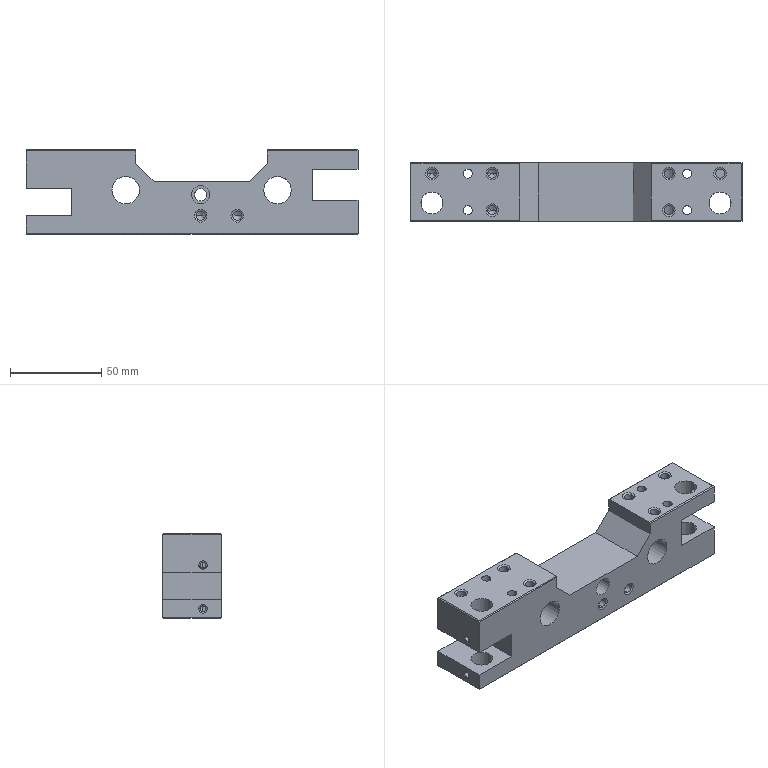Part | NX | 1 solid | 115 faces | box 181.5 x 32 x 46 mm | volume 178002 mm3 | cylinder 48 | cone 36 | plane 31 | commonest cylinder face diameters 5 x24 3.3 x8 12 x8 15 x4 6.8 x2 10 x2